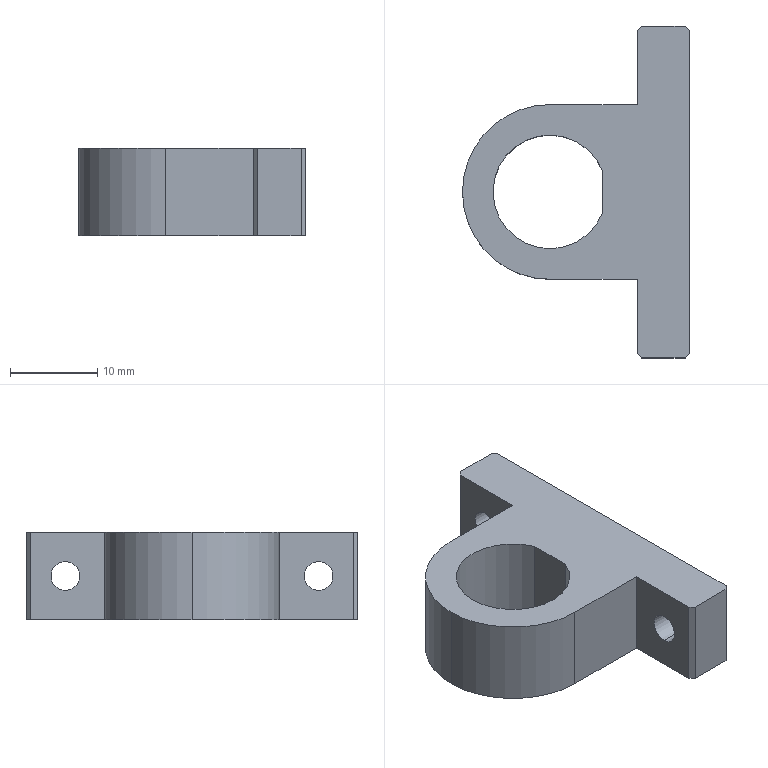Part | STEP file | slide seat | 1 solid | 22 faces | box 26 x 38 x 10 mm | volume 4433 mm3 | plane 14 | cylinder 8 | commonest cylinder face diameters 3.3 x4 13 x2 20 x2